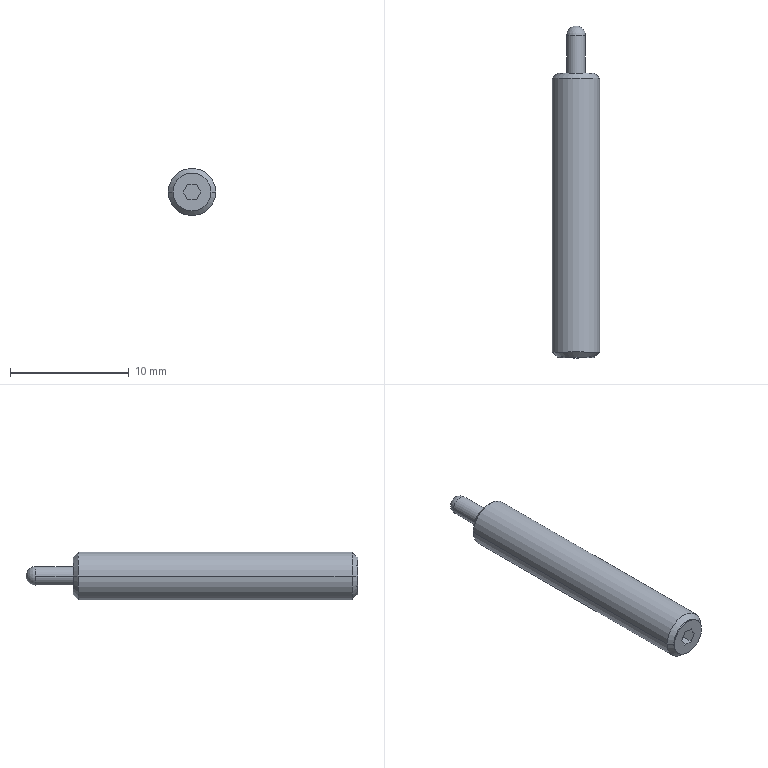Part | NX | 1 solid | 20 faces | box 4 x 28 x 4 mm | volume 304.868 mm3 | plane 9 | cylinder 6 | cone 4 | sphere 1 | commonest cylinder face diameters 1.6 x2 3.2 x2 4 x2
STEP:
#1=CARTESIAN_POINT('',(-0.8,27.2,0.));
#2=VERTEX_POINT('',#1);
#3=CARTESIAN_POINT('',(0.8,27.2,0.));
#4=VERTEX_POINT('',#3);
#5=CARTESIAN_POINT('',(0.,27.2,0.));
#6=DIRECTION('',(0.,1.,0.));
#7=DIRECTION('',(1.,0.,0.));
#8=AXIS2_PLACEMENT_3D('',#5,#6,#7);
#9=CIRCLE('',#8,0.8);
#10=EDGE_CURVE('',#2,#4,#9,.T.);
#11=ORIENTED_EDGE('',*,*,#10,.T.);
#12=CARTESIAN_POINT('',(0.,27.2,0.));
#13=DIRECTION('',(0.,1.,0.));
#14=DIRECTION('',(1.,0.,0.));
#15=AXIS2_PLACEMENT_3D('',#12,#13,#14);
#16=CIRCLE('',#15,0.8);
#17=EDGE_CURVE('',#4,#2,#16,.T.);
#18=ORIENTED_EDGE('',*,*,#17,.T.);
#19=EDGE_LOOP('',(#11,#18));
#20=FACE_BOUND('',#19,.T.);
#21=CARTESIAN_POINT('',(0.,27.2,0.));
#22=DIRECTION('',(0.,1.,0.));
#23=DIRECTION('',(1.,0.,0.));
#24=AXIS2_PLACEMENT_3D('',#21,#22,#23);
#25=SPHERICAL_SURFACE('',#24,0.8);
#26=ADVANCED_FACE('',(#20),#25,.T.);
#27=CARTESIAN_POINT('',(0.3753,1.3,0.65));
#28=VERTEX_POINT('',#27);
#29=CARTESIAN_POINT('',(0.7506,1.3,0.));
#30=VERTEX_POINT('',#29);
#31=CARTESIAN_POINT('',(0.3753,1.3,0.65));
#32=DIRECTION('',(0.5,0.,-0.866));
#33=VECTOR('',#32,1000.);
#34=LINE('',#31,#33);
#35=EDGE_CURVE('',#28,#30,#34,.T.);
#36=ORIENTED_EDGE('',*,*,#35,.F.);
#37=CARTESIAN_POINT('',(-0.3753,1.3,0.65));
#38=VERTEX_POINT('',#37);
#39=CARTESIAN_POINT('',(-0.3753,1.3,0.65));
#40=DIRECTION('',(1.,0.,0.));
#41=VECTOR('',#40,1000.);
#42=LINE('',#39,#41);
#43=EDGE_CURVE('',#38,#28,#42,.T.);
#44=ORIENTED_EDGE('',*,*,#43,.F.);
#45=CARTESIAN_POINT('',(-0.7506,1.3,0.));
#46=VERTEX_POINT('',#45);
#47=CARTESIAN_POINT('',(-0.7506,1.3,0.));
#48=DIRECTION('',(0.5,0.,0.866));
#49=VECTOR('',#48,1000.);
#50=LINE('',#47,#49);
#51=EDGE_CURVE('',#46,#38,#50,.T.);
#52=ORIENTED_EDGE('',*,*,#51,.F.);
#53=CARTESIAN_POINT('',(-0.3753,1.3,-0.65));
#54=VERTEX_POINT('',#53);
#55=CARTESIAN_POINT('',(-0.3753,1.3,-0.65));
#56=DIRECTION('',(-0.5,0.,0.866));
#57=VECTOR('',#56,1000.);
#58=LINE('',#55,#57);
#59=EDGE_CURVE('',#54,#46,#58,.T.);
#60=ORIENTED_EDGE('',*,*,#59,.F.);
#61=CARTESIAN_POINT('',(0.3753,1.3,-0.65));
#62=VERTEX_POINT('',#61);
#63=CARTESIAN_POINT('',(0.3753,1.3,-0.65));
#64=DIRECTION('',(-1.,0.,0.));
#65=VECTOR('',#64,1000.);
#66=LINE('',#63,#65);
#67=EDGE_CURVE('',#62,#54,#66,.T.);
#68=ORIENTED_EDGE('',*,*,#67,.F.);
#69=CARTESIAN_POINT('',(0.7506,1.3,0.));
#70=DIRECTION('',(-0.5,0.,-0.866));
#71=VECTOR('',#70,1000.);
#72=LINE('',#69,#71);
#73=EDGE_CURVE('',#30,#62,#72,.T.);
#74=ORIENTED_EDGE('',*,*,#73,.F.);
#75=EDGE_LOOP('',(#36,#44,#52,#60,#68,#74));
#76=FACE_BOUND('',#75,.T.);
#77=CARTESIAN_POINT('',(0.,1.3,0.));
#78=DIRECTION('',(0.,-1.,0.));
#79=DIRECTION('',(0.,0.,-1.));
#80=AXIS2_PLACEMENT_3D('',#77,#78,#79);
#81=PLANE('',#80);
#82=ADVANCED_FACE('',(#76),#81,.T.);
#83=ORIENTED_EDGE('',*,*,#17,.F.);
#84=CARTESIAN_POINT('',(0.8,24.,0.));
#85=VERTEX_POINT('',#84);
#86=CARTESIAN_POINT('',(0.8,29.4,0.));
#87=DIRECTION('',(0.,-1.,0.));
#88=VECTOR('',#87,1000.);
#89=LINE('',#86,#88);
#90=EDGE_CURVE('',#4,#85,#89,.T.);
#91=ORIENTED_EDGE('',*,*,#90,.T.);
#92=CARTESIAN_POINT('',(-0.8,24.,0.));
#93=VERTEX_POINT('',#92);
#94=CARTESIAN_POINT('',(0.,24.,0.));
#95=DIRECTION('',(0.,1.,0.));
#96=DIRECTION('',(1.,0.,0.));
#97=AXIS2_PLACEMENT_3D('',#94,#95,#96);
#98=CIRCLE('',#97,0.8);
#99=EDGE_CURVE('',#85,#93,#98,.T.);
#100=ORIENTED_EDGE('',*,*,#99,.T.);
#101=CARTESIAN_POINT('',(-0.8,29.4,0.));
#102=DIRECTION('',(0.,-1.,0.));
#103=VECTOR('',#102,1000.);
#104=LINE('',#101,#103);
#105=EDGE_CURVE('',#2,#93,#104,.T.);
#106=ORIENTED_EDGE('',*,*,#105,.F.);
#107=EDGE_LOOP('',(#83,#91,#100,#106));
#108=FACE_BOUND('',#107,.T.);
#109=CARTESIAN_POINT('',(0.,29.4,0.));
#110=DIRECTION('',(0.,-1.,0.));
#111=DIRECTION('',(-1.,0.,0.));
#112=AXIS2_PLACEMENT_3D('',#109,#110,#111);
#113=CYLINDRICAL_SURFACE('',#112,0.8);
#114=ADVANCED_FACE('',(#108),#113,.T.);
#115=CARTESIAN_POINT('',(0.3753,0.,-0.65));
#116=VERTEX_POINT('',#115);
#117=CARTESIAN_POINT('',(-0.3753,0.,-0.65));
#118=VERTEX_POINT('',#117);
#119=CARTESIAN_POINT('',(0.3753,0.,-0.65));
#120=DIRECTION('',(-1.,0.,0.));
#121=VECTOR('',#120,1000.);
#122=LINE('',#119,#121);
#123=EDGE_CURVE('',#116,#118,#122,.T.);
#124=ORIENTED_EDGE('',*,*,#123,.F.);
#125=CARTESIAN_POINT('',(0.3753,1.3,-0.65));
#126=DIRECTION('',(0.,-1.,0.));
#127=VECTOR('',#126,1000.);
#128=LINE('',#125,#127);
#129=EDGE_CURVE('',#62,#116,#128,.T.);
#130=ORIENTED_EDGE('',*,*,#129,.F.);
#131=ORIENTED_EDGE('',*,*,#67,.T.);
#132=CARTESIAN_POINT('',(-0.3753,1.3,-0.65));
#133=DIRECTION('',(0.,-1.,0.));
#134=VECTOR('',#133,1000.);
#135=LINE('',#132,#134);
#136=EDGE_CURVE('',#54,#118,#135,.T.);
#137=ORIENTED_EDGE('',*,*,#136,.T.);
#138=EDGE_LOOP('',(#124,#130,#131,#137));
#139=FACE_BOUND('',#138,.T.);
#140=CARTESIAN_POINT('',(-0.3753,0.,-0.65));
#141=DIRECTION('',(0.,0.,-1.));
#142=DIRECTION('',(0.,-1.,0.));
#143=AXIS2_PLACEMENT_3D('',#140,#141,#142);
#144=PLANE('',#143);
#145=ADVANCED_FACE('',(#139),#144,.F.);
#146=CARTESIAN_POINT('',(1.6,24.,0.));
#147=VERTEX_POINT('',#146);
#148=CARTESIAN_POINT('',(-1.6,24.,0.));
#149=VERTEX_POINT('',#148);
#150=CARTESIAN_POINT('',(0.,24.,0.));
#151=DIRECTION('',(0.,-1.,0.));
#152=DIRECTION('',(-1.,0.,0.));
#153=AXIS2_PLACEMENT_3D('',#150,#151,#152);
#154=CIRCLE('',#153,1.6);
#155=EDGE_CURVE('',#147,#149,#154,.T.);
#156=ORIENTED_EDGE('',*,*,#155,.F.);
#157=CARTESIAN_POINT('',(0.,24.,0.));
#158=DIRECTION('',(0.,-1.,0.));
#159=DIRECTION('',(-1.,0.,0.));
#160=AXIS2_PLACEMENT_3D('',#157,#158,#159);
#161=CIRCLE('',#160,1.6);
#162=EDGE_CURVE('',#149,#147,#161,.T.);
#163=ORIENTED_EDGE('',*,*,#162,.F.);
#164=EDGE_LOOP('',(#156,#163));
#165=FACE_BOUND('',#164,.T.);
#166=CARTESIAN_POINT('',(0.,24.,0.));
#167=DIRECTION('',(0.,1.,0.));
#168=DIRECTION('',(1.,0.,0.));
#169=AXIS2_PLACEMENT_3D('',#166,#167,#168);
#170=CIRCLE('',#169,0.8);
#171=EDGE_CURVE('',#93,#85,#170,.T.);
#172=ORIENTED_EDGE('',*,*,#171,.F.);
#173=ORIENTED_EDGE('',*,*,#99,.F.);
#174=EDGE_LOOP('',(#172,#173));
#175=FACE_BOUND('',#174,.T.);
#176=CARTESIAN_POINT('',(0.,24.,0.));
#177=DIRECTION('',(0.,-1.,0.));
#178=DIRECTION('',(0.,0.,-1.));
#179=AXIS2_PLACEMENT_3D('',#176,#177,#178);
#180=PLANE('',#179);
#181=ADVANCED_FACE('',(#165,#175),#180,.F.);
#182=CARTESIAN_POINT('',(-2.,23.6,0.));
#183=VERTEX_POINT('',#182);
#184=CARTESIAN_POINT('',(2.,23.6,0.));
#185=VERTEX_POINT('',#184);
#186=CARTESIAN_POINT('',(0.,23.6,0.));
#187=DIRECTION('',(0.,-1.,0.));
#188=DIRECTION('',(1.,0.,0.));
#189=AXIS2_PLACEMENT_3D('',#186,#187,#188);
#190=CIRCLE('',#189,2.);
#191=EDGE_CURVE('',#183,#185,#190,.T.);
#192=ORIENTED_EDGE('',*,*,#191,.F.);
#193=CARTESIAN_POINT('',(-1.8,23.8,0.));
#194=DIRECTION('',(-0.7071,-0.7071,0.));
#195=VECTOR('',#194,1000.);
#196=LINE('',#193,#195);
#197=EDGE_CURVE('',#183,#149,#196,.F.);
#198=ORIENTED_EDGE('',*,*,#197,.T.);
#199=ORIENTED_EDGE('',*,*,#162,.T.);
#200=CARTESIAN_POINT('',(1.8,23.8,0.));
#201=DIRECTION('',(0.7071,-0.7071,0.));
#202=VECTOR('',#201,1000.);
#203=LINE('',#200,#202);
#204=EDGE_CURVE('',#185,#147,#203,.F.);
#205=ORIENTED_EDGE('',*,*,#204,.F.);
#206=EDGE_LOOP('',(#192,#198,#199,#205));
#207=FACE_BOUND('',#206,.T.);
#208=CARTESIAN_POINT('',(0.,23.8,0.));
#209=DIRECTION('',(0.,-1.,0.));
#210=DIRECTION('',(-1.,0.,0.));
#211=AXIS2_PLACEMENT_3D('',#208,#209,#210);
#212=CONICAL_SURFACE('',#211,1.8,0.7854);
#213=ADVANCED_FACE('',(#207),#212,.T.);
#214=CARTESIAN_POINT('',(-0.3753,0.,0.65));
#215=VERTEX_POINT('',#214);
#216=CARTESIAN_POINT('',(-0.7506,0.,0.));
#217=VERTEX_POINT('',#216);
#218=CARTESIAN_POINT('',(-0.3753,0.,0.65));
#219=DIRECTION('',(-0.5,0.,-0.866));
#220=VECTOR('',#219,1000.);
#221=LINE('',#218,#220);
#222=EDGE_CURVE('',#215,#217,#221,.T.);
#223=ORIENTED_EDGE('',*,*,#222,.T.);
#224=CARTESIAN_POINT('',(-0.7506,1.3,0.));
#225=DIRECTION('',(0.,-1.,0.));
#226=VECTOR('',#225,1000.);
#227=LINE('',#224,#226);
#228=EDGE_CURVE('',#46,#217,#227,.T.);
#229=ORIENTED_EDGE('',*,*,#228,.F.);
#230=ORIENTED_EDGE('',*,*,#51,.T.);
#231=CARTESIAN_POINT('',(-0.3753,1.3,0.65));
#232=DIRECTION('',(0.,-1.,0.));
#233=VECTOR('',#232,1000.);
#234=LINE('',#231,#233);
#235=EDGE_CURVE('',#38,#215,#234,.T.);
#236=ORIENTED_EDGE('',*,*,#235,.T.);
#237=EDGE_LOOP('',(#223,#229,#230,#236));
#238=FACE_BOUND('',#237,.T.);
#239=CARTESIAN_POINT('',(-0.3753,0.,0.65));
#240=DIRECTION('',(-0.866,0.,0.5));
#241=DIRECTION('',(0.,1.,0.));
#242=AXIS2_PLACEMENT_3D('',#239,#240,#241);
#243=PLANE('',#242);
#244=ADVANCED_FACE('',(#238),#243,.F.);
#245=ORIENTED_EDGE('',*,*,#191,.T.);
#246=CARTESIAN_POINT('',(2.,0.5,0.));
#247=VERTEX_POINT('',#246);
#248=CARTESIAN_POINT('',(2.,29.4,0.));
#249=DIRECTION('',(0.,-1.,0.));
#250=VECTOR('',#249,1000.);
#251=LINE('',#248,#250);
#252=EDGE_CURVE('',#185,#247,#251,.T.);
#253=ORIENTED_EDGE('',*,*,#252,.T.);
#254=CARTESIAN_POINT('',(-2.,0.5,0.));
#255=VERTEX_POINT('',#254);
#256=CARTESIAN_POINT('',(0.,0.5,0.));
#257=DIRECTION('',(0.,1.,0.));
#258=DIRECTION('',(1.,0.,0.));
#259=AXIS2_PLACEMENT_3D('',#256,#257,#258);
#260=CIRCLE('',#259,2.);
#261=EDGE_CURVE('',#247,#255,#260,.T.);
#262=ORIENTED_EDGE('',*,*,#261,.T.);
#263=CARTESIAN_POINT('',(-2.,29.4,0.));
#264=DIRECTION('',(0.,-1.,0.));
#265=VECTOR('',#264,1000.);
#266=LINE('',#263,#265);
#267=EDGE_CURVE('',#183,#255,#266,.T.);
#268=ORIENTED_EDGE('',*,*,#267,.F.);
#269=EDGE_LOOP('',(#245,#253,#262,#268));
#270=FACE_BOUND('',#269,.T.);
#271=CARTESIAN_POINT('',(0.,29.4,0.));
#272=DIRECTION('',(0.,-1.,0.));
#273=DIRECTION('',(-1.,0.,0.));
#274=AXIS2_PLACEMENT_3D('',#271,#272,#273);
#275=CYLINDRICAL_SURFACE('',#274,2.);
#276=ADVANCED_FACE('',(#270),#275,.T.);
#277=CARTESIAN_POINT('',(0.7506,0.,0.));
#278=VERTEX_POINT('',#277);
#279=CARTESIAN_POINT('',(0.3753,0.,-0.65));
#280=DIRECTION('',(0.5,0.,0.866));
#281=VECTOR('',#280,1000.);
#282=LINE('',#279,#281);
#283=EDGE_CURVE('',#116,#278,#282,.T.);
#284=ORIENTED_EDGE('',*,*,#283,.T.);
#285=CARTESIAN_POINT('',(0.7506,1.3,0.));
#286=DIRECTION('',(0.,-1.,0.));
#287=VECTOR('',#286,1000.);
#288=LINE('',#285,#287);
#289=EDGE_CURVE('',#30,#278,#288,.T.);
#290=ORIENTED_EDGE('',*,*,#289,.F.);
#291=ORIENTED_EDGE('',*,*,#73,.T.);
#292=ORIENTED_EDGE('',*,*,#129,.T.);
#293=EDGE_LOOP('',(#284,#290,#291,#292));
#294=FACE_BOUND('',#293,.T.);
#295=CARTESIAN_POINT('',(0.3753,0.,-0.65));
#296=DIRECTION('',(0.866,0.,-0.5));
#297=DIRECTION('',(0.,-1.,0.));
#298=AXIS2_PLACEMENT_3D('',#295,#296,#297);
#299=PLANE('',#298);
#300=ADVANCED_FACE('',(#294),#299,.F.);
#301=CARTESIAN_POINT('',(1.6,0.1,0.));
#302=VERTEX_POINT('',#301);
#303=CARTESIAN_POINT('',(-1.6,0.1,0.));
#304=VERTEX_POINT('',#303);
#305=CARTESIAN_POINT('',(0.,0.1,0.));
#306=DIRECTION('',(0.,-1.,0.));
#307=DIRECTION('',(-1.,0.,0.));
#308=AXIS2_PLACEMENT_3D('',#305,#306,#307);
#309=CIRCLE('',#308,1.6);
#310=EDGE_CURVE('',#302,#304,#309,.T.);
#311=ORIENTED_EDGE('',*,*,#310,.F.);
#312=CARTESIAN_POINT('',(1.8,0.3,0.));
#313=DIRECTION('',(0.7071,0.7071,0.));
#314=VECTOR('',#313,1000.);
#315=LINE('',#312,#314);
#316=EDGE_CURVE('',#302,#247,#315,.T.);
#317=ORIENTED_EDGE('',*,*,#316,.T.);
#318=CARTESIAN_POINT('',(0.,0.5,0.));
#319=DIRECTION('',(0.,1.,0.));
#320=DIRECTION('',(1.,0.,0.));
#321=AXIS2_PLACEMENT_3D('',#318,#319,#320);
#322=CIRCLE('',#321,2.);
#323=EDGE_CURVE('',#255,#247,#322,.T.);
#324=ORIENTED_EDGE('',*,*,#323,.F.);
#325=CARTESIAN_POINT('',(-1.8,0.3,0.));
#326=DIRECTION('',(-0.7071,0.7071,0.));
#327=VECTOR('',#326,1000.);
#328=LINE('',#325,#327);
#329=EDGE_CURVE('',#304,#255,#328,.T.);
#330=ORIENTED_EDGE('',*,*,#329,.F.);
#331=EDGE_LOOP('',(#311,#317,#324,#330));
#332=FACE_BOUND('',#331,.T.);
#333=CARTESIAN_POINT('',(0.,0.3,0.));
#334=DIRECTION('',(0.,1.,0.));
#335=DIRECTION('',(1.,0.,0.));
#336=AXIS2_PLACEMENT_3D('',#333,#334,#335);
#337=CONICAL_SURFACE('',#336,1.8,0.7854);
#338=ADVANCED_FACE('',(#332),#337,.T.);
#339=CARTESIAN_POINT('',(-0.7506,0.,0.));
#340=DIRECTION('',(0.5,0.,-0.866));
#341=VECTOR('',#340,1000.);
#342=LINE('',#339,#341);
#343=EDGE_CURVE('',#217,#118,#342,.T.);
#344=ORIENTED_EDGE('',*,*,#343,.T.);
#345=ORIENTED_EDGE('',*,*,#136,.F.);
#346=ORIENTED_EDGE('',*,*,#59,.T.);
#347=ORIENTED_EDGE('',*,*,#228,.T.);
#348=EDGE_LOOP('',(#344,#345,#346,#347));
#349=FACE_BOUND('',#348,.T.);
#350=CARTESIAN_POINT('',(-0.7506,0.,0.));
#351=DIRECTION('',(-0.866,0.,-0.5));
#352=DIRECTION('',(-0.5,0.,0.866));
#353=AXIS2_PLACEMENT_3D('',#350,#351,#352);
#354=PLANE('',#353);
#355=ADVANCED_FACE('',(#349),#354,.F.);
#356=CARTESIAN_POINT('',(-1.6,0.,0.));
#357=VERTEX_POINT('',#356);
#358=CARTESIAN_POINT('',(1.6,0.,0.));
#359=VERTEX_POINT('',#358);
#360=CARTESIAN_POINT('',(0.,0.,0.));
#361=DIRECTION('',(0.,1.,0.));
#362=DIRECTION('',(1.,0.,0.));
#363=AXIS2_PLACEMENT_3D('',#360,#361,#362);
#364=CIRCLE('',#363,1.6);
#365=EDGE_CURVE('',#357,#359,#364,.T.);
#366=ORIENTED_EDGE('',*,*,#365,.T.);
#367=CARTESIAN_POINT('',(1.6,29.4,0.));
#368=DIRECTION('',(0.,-1.,0.));
#369=VECTOR('',#368,1000.);
#370=LINE('',#367,#369);
#371=EDGE_CURVE('',#359,#302,#370,.F.);
#372=ORIENTED_EDGE('',*,*,#371,.T.);
#373=ORIENTED_EDGE('',*,*,#310,.T.);
#374=CARTESIAN_POINT('',(-1.6,29.4,0.));
#375=DIRECTION('',(0.,-1.,0.));
#376=VECTOR('',#375,1000.);
#377=LINE('',#374,#376);
#378=EDGE_CURVE('',#357,#304,#377,.F.);
#379=ORIENTED_EDGE('',*,*,#378,.F.);
#380=EDGE_LOOP('',(#366,#372,#373,#379));
#381=FACE_BOUND('',#380,.T.);
#382=CARTESIAN_POINT('',(0.,29.4,0.));
#383=DIRECTION('',(0.,-1.,0.));
#384=DIRECTION('',(-1.,0.,0.));
#385=AXIS2_PLACEMENT_3D('',#382,#383,#384);
#386=CYLINDRICAL_SURFACE('',#385,1.6);
#387=ADVANCED_FACE('',(#381),#386,.T.);
#388=CARTESIAN_POINT('',(0.3753,0.,0.65));
#389=VERTEX_POINT('',#388);
#390=CARTESIAN_POINT('',(-0.3753,0.,0.65));
#391=DIRECTION('',(1.,0.,0.));
#392=VECTOR('',#391,1000.);
#393=LINE('',#390,#392);
#394=EDGE_CURVE('',#215,#389,#393,.T.);
#395=ORIENTED_EDGE('',*,*,#394,.F.);
#396=ORIENTED_EDGE('',*,*,#235,.F.);
#397=ORIENTED_EDGE('',*,*,#43,.T.);
#398=CARTESIAN_POINT('',(0.3753,1.3,0.65));
#399=DIRECTION('',(0.,-1.,0.));
#400=VECTOR('',#399,1000.);
#401=LINE('',#398,#400);
#402=EDGE_CURVE('',#28,#389,#401,.T.);
#403=ORIENTED_EDGE('',*,*,#402,.T.);
#404=EDGE_LOOP('',(#395,#396,#397,#403));
#405=FACE_BOUND('',#404,.T.);
#406=CARTESIAN_POINT('',(0.3753,0.,0.65));
#407=DIRECTION('',(0.,0.,1.));
#408=DIRECTION('',(1.,0.,0.));
#409=AXIS2_PLACEMENT_3D('',#406,#407,#408);
#410=PLANE('',#409);
#411=ADVANCED_FACE('',(#405),#410,.F.);
#412=ORIENTED_EDGE('',*,*,#365,.F.);
#413=CARTESIAN_POINT('',(0.,0.,0.));
#414=DIRECTION('',(0.,1.,0.));
#415=DIRECTION('',(1.,0.,0.));
#416=AXIS2_PLACEMENT_3D('',#413,#414,#415);
#417=CIRCLE('',#416,1.6);
#418=EDGE_CURVE('',#359,#357,#417,.T.);
#419=ORIENTED_EDGE('',*,*,#418,.F.);
#420=EDGE_LOOP('',(#412,#419));
#421=FACE_BOUND('',#420,.T.);
#422=CARTESIAN_POINT('',(0.7506,0.,0.));
#423=DIRECTION('',(-0.5,0.,0.866));
#424=VECTOR('',#423,1000.);
#425=LINE('',#422,#424);
#426=EDGE_CURVE('',#278,#389,#425,.T.);
#427=ORIENTED_EDGE('',*,*,#426,.F.);
#428=ORIENTED_EDGE('',*,*,#283,.F.);
#429=ORIENTED_EDGE('',*,*,#123,.T.);
#430=ORIENTED_EDGE('',*,*,#343,.F.);
#431=ORIENTED_EDGE('',*,*,#222,.F.);
#432=ORIENTED_EDGE('',*,*,#394,.T.);
#433=EDGE_LOOP('',(#427,#428,#429,#430,#431,#432));
#434=FACE_BOUND('',#433,.T.);
#435=CARTESIAN_POINT('',(0.,0.,0.));
#436=DIRECTION('',(0.,-1.,0.));
#437=DIRECTION('',(0.,0.,-1.));
#438=AXIS2_PLACEMENT_3D('',#435,#436,#437);
#439=PLANE('',#438);
#440=ADVANCED_FACE('',(#421,#434),#439,.T.);
#441=ORIENTED_EDGE('',*,*,#426,.T.);
#442=ORIENTED_EDGE('',*,*,#402,.F.);
#443=ORIENTED_EDGE('',*,*,#35,.T.);
#444=ORIENTED_EDGE('',*,*,#289,.T.);
#445=EDGE_LOOP('',(#441,#442,#443,#444));
#446=FACE_BOUND('',#445,.T.);
#447=CARTESIAN_POINT('',(0.7506,0.,0.));
#448=DIRECTION('',(0.866,0.,0.5));
#449=DIRECTION('',(0.,-1.,0.));
#450=AXIS2_PLACEMENT_3D('',#447,#448,#449);
#451=PLANE('',#450);
#452=ADVANCED_FACE('',(#446),#451,.F.);
#453=ORIENTED_EDGE('',*,*,#378,.T.);
#454=CARTESIAN_POINT('',(0.,0.1,0.));
#455=DIRECTION('',(0.,-1.,0.));
#456=DIRECTION('',(-1.,0.,0.));
#457=AXIS2_PLACEMENT_3D('',#454,#455,#456);
#458=CIRCLE('',#457,1.6);
#459=EDGE_CURVE('',#304,#302,#458,.T.);
#460=ORIENTED_EDGE('',*,*,#459,.T.);
#461=ORIENTED_EDGE('',*,*,#371,.F.);
#462=ORIENTED_EDGE('',*,*,#418,.T.);
#463=EDGE_LOOP('',(#453,#460,#461,#462));
#464=FACE_BOUND('',#463,.T.);
#465=CARTESIAN_POINT('',(0.,29.4,0.));
#466=DIRECTION('',(0.,-1.,0.));
#467=DIRECTION('',(-1.,0.,0.));
#468=AXIS2_PLACEMENT_3D('',#465,#466,#467);
#469=CYLINDRICAL_SURFACE('',#468,1.6);
#470=ADVANCED_FACE('',(#464),#469,.T.);
#471=ORIENTED_EDGE('',*,*,#316,.F.);
#472=ORIENTED_EDGE('',*,*,#459,.F.);
#473=ORIENTED_EDGE('',*,*,#329,.T.);
#474=ORIENTED_EDGE('',*,*,#261,.F.);
#475=EDGE_LOOP('',(#471,#472,#473,#474));
#476=FACE_BOUND('',#475,.T.);
#477=CARTESIAN_POINT('',(0.,0.3,0.));
#478=DIRECTION('',(0.,1.,0.));
#479=DIRECTION('',(1.,0.,0.));
#480=AXIS2_PLACEMENT_3D('',#477,#478,#479);
#481=CONICAL_SURFACE('',#480,1.8,0.7854);
#482=ADVANCED_FACE('',(#476),#481,.T.);
#483=ORIENTED_EDGE('',*,*,#323,.T.);
#484=ORIENTED_EDGE('',*,*,#252,.F.);
#485=CARTESIAN_POINT('',(0.,23.6,0.));
#486=DIRECTION('',(0.,-1.,0.));
#487=DIRECTION('',(1.,0.,0.));
#488=AXIS2_PLACEMENT_3D('',#485,#486,#487);
#489=CIRCLE('',#488,2.);
#490=EDGE_CURVE('',#185,#183,#489,.T.);
#491=ORIENTED_EDGE('',*,*,#490,.T.);
#492=ORIENTED_EDGE('',*,*,#267,.T.);
#493=EDGE_LOOP('',(#483,#484,#491,#492));
#494=FACE_BOUND('',#493,.T.);
#495=CARTESIAN_POINT('',(0.,29.4,0.));
#496=DIRECTION('',(0.,-1.,0.));
#497=DIRECTION('',(-1.,0.,0.));
#498=AXIS2_PLACEMENT_3D('',#495,#496,#497);
#499=CYLINDRICAL_SURFACE('',#498,2.);
#500=ADVANCED_FACE('',(#494),#499,.T.);
#501=ORIENTED_EDGE('',*,*,#155,.T.);
#502=ORIENTED_EDGE('',*,*,#197,.F.);
#503=ORIENTED_EDGE('',*,*,#490,.F.);
#504=ORIENTED_EDGE('',*,*,#204,.T.);
#505=EDGE_LOOP('',(#501,#502,#503,#504));
#506=FACE_BOUND('',#505,.T.);
#507=CARTESIAN_POINT('',(0.,23.8,0.));
#508=DIRECTION('',(0.,-1.,0.));
#509=DIRECTION('',(-1.,0.,0.));
#510=AXIS2_PLACEMENT_3D('',#507,#508,#509);
#511=CONICAL_SURFACE('',#510,1.8,0.7854);
#512=ADVANCED_FACE('',(#506),#511,.T.);
#513=ORIENTED_EDGE('',*,*,#171,.T.);
#514=ORIENTED_EDGE('',*,*,#90,.F.);
#515=ORIENTED_EDGE('',*,*,#10,.F.);
#516=ORIENTED_EDGE('',*,*,#105,.T.);
#517=EDGE_LOOP('',(#513,#514,#515,#516));
#518=FACE_BOUND('',#517,.T.);
#519=CARTESIAN_POINT('',(0.,29.4,0.));
#520=DIRECTION('',(0.,-1.,0.));
#521=DIRECTION('',(-1.,0.,0.));
#522=AXIS2_PLACEMENT_3D('',#519,#520,#521);
#523=CYLINDRICAL_SURFACE('',#522,0.8);
#524=ADVANCED_FACE('',(#518),#523,.T.);
#525=CLOSED_SHELL('',(#26,#82,#114,#145,#181,#213,#244,#276,#300,#338,#355,#387,#411,#440,#452,#470,#482,#500,#512,#524));
#526=MANIFOLD_SOLID_BREP('',#525);
#527=(LENGTH_UNIT()NAMED_UNIT(*)SI_UNIT(.MILLI.,.METRE.));
#528=UNCERTAINTY_MEASURE_WITH_UNIT(LENGTH_MEASURE(0.00001),#527,'','');
#529=(NAMED_UNIT(*)PLANE_ANGLE_UNIT()SI_UNIT($,.RADIAN.));
#530=(NAMED_UNIT(*)SI_UNIT($,.STERADIAN.)SOLID_ANGLE_UNIT());
#531=(GEOMETRIC_REPRESENTATION_CONTEXT(3)GLOBAL_UNCERTAINTY_ASSIGNED_CONTEXT((#528))GLOBAL_UNIT_ASSIGNED_CONTEXT((#527,#529,#530))REPRESENTATION_CONTEXT('',''));
#532=ADVANCED_BREP_SHAPE_REPRESENTATION('',(#526),#531);